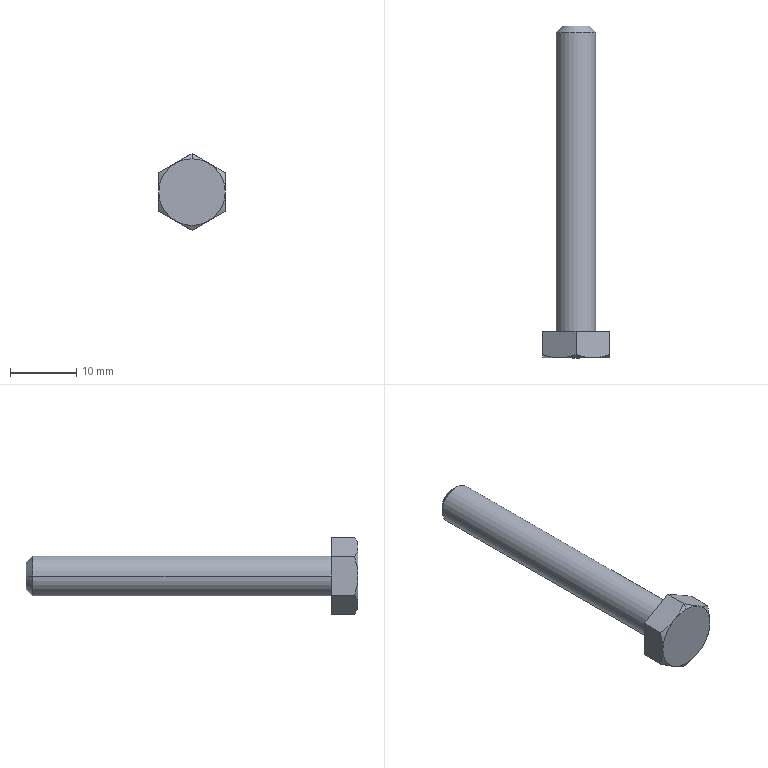Part | STEP file | 11-NEZI-M6x40L_MC01-S311 | 1 solid | 20 faces | box 10 x 50 x 11.547 mm | volume 1637 mm3 | cone 9 | plane 9 | cylinder 2 | commonest cylinder face diameters 6 x2
STEP:
#1=CARTESIAN_POINT('',(-2.,50.,0.));
#2=VERTEX_POINT('',#1);
#3=CARTESIAN_POINT('',(2.,50.,0.));
#4=VERTEX_POINT('',#3);
#5=CARTESIAN_POINT('',(0.,50.,0.));
#6=DIRECTION('',(0.,1.,0.));
#7=DIRECTION('',(-1.,0.,0.));
#8=AXIS2_PLACEMENT_3D('',#5,#6,#7);
#9=CIRCLE('',#8,2.);
#10=EDGE_CURVE('',#2,#4,#9,.T.);
#11=ORIENTED_EDGE('',*,*,#10,.F.);
#12=CARTESIAN_POINT('',(-3.,49.,0.));
#13=VERTEX_POINT('',#12);
#14=CARTESIAN_POINT('',(-2.,50.,0.));
#15=DIRECTION('',(-0.7071,-0.7071,0.));
#16=VECTOR('',#15,1000.);
#17=LINE('',#14,#16);
#18=EDGE_CURVE('',#2,#13,#17,.T.);
#19=ORIENTED_EDGE('',*,*,#18,.T.);
#20=CARTESIAN_POINT('',(3.,49.,0.));
#21=VERTEX_POINT('',#20);
#22=CARTESIAN_POINT('',(0.,49.,0.));
#23=DIRECTION('',(0.,-1.,0.));
#24=DIRECTION('',(-1.,0.,0.));
#25=AXIS2_PLACEMENT_3D('',#22,#23,#24);
#26=CIRCLE('',#25,3.);
#27=EDGE_CURVE('',#21,#13,#26,.T.);
#28=ORIENTED_EDGE('',*,*,#27,.F.);
#29=CARTESIAN_POINT('',(2.,50.,0.));
#30=DIRECTION('',(0.7071,-0.7071,0.));
#31=VECTOR('',#30,1000.);
#32=LINE('',#29,#31);
#33=EDGE_CURVE('',#4,#21,#32,.T.);
#34=ORIENTED_EDGE('',*,*,#33,.F.);
#35=EDGE_LOOP('',(#11,#19,#28,#34));
#36=FACE_OUTER_BOUND('',#35,.T.);
#37=CARTESIAN_POINT('',(0.,50.,0.));
#38=DIRECTION('',(0.,-1.,0.));
#39=DIRECTION('',(1.,0.,0.));
#40=AXIS2_PLACEMENT_3D('',#37,#38,#39);
#41=CONICAL_SURFACE('',#40,2.,0.7854);
#42=ADVANCED_FACE('',(#36),#41,.T.);
#43=CARTESIAN_POINT('',(0.,0.,5.));
#44=VERTEX_POINT('',#43);
#45=CARTESIAN_POINT('',(-2.5,0.,4.33));
#46=VERTEX_POINT('',#45);
#47=CARTESIAN_POINT('',(0.,0.,0.));
#48=DIRECTION('',(0.,-1.,0.));
#49=DIRECTION('',(1.,0.,0.));
#50=AXIS2_PLACEMENT_3D('',#47,#48,#49);
#51=CIRCLE('',#50,5.);
#52=EDGE_CURVE('',#44,#46,#51,.T.);
#53=ORIENTED_EDGE('',*,*,#52,.F.);
#54=CARTESIAN_POINT('',(0.,0.5,5.774));
#55=VERTEX_POINT('',#54);
#56=CARTESIAN_POINT('',(0.,0.,5.));
#57=DIRECTION('',(0.,0.5429,0.8398));
#58=VECTOR('',#57,1000.);
#59=LINE('',#56,#58);
#60=EDGE_CURVE('',#44,#55,#59,.T.);
#61=ORIENTED_EDGE('',*,*,#60,.T.);
#62=CARTESIAN_POINT('',(0.,0.5,5.774));
#63=CARTESIAN_POINT('',(-0.8145,0.196,5.303));
#64=CARTESIAN_POINT('',(-1.644,0.,4.824));
#65=CARTESIAN_POINT('',(-2.5,0.,4.33));
#66=B_SPLINE_CURVE_WITH_KNOTS('',3,(#62,#63,#64,#65),.UNSPECIFIED.,.F.,.F.,(4,4),(0.00000024,0.00293),.UNSPECIFIED.);
#67=EDGE_CURVE('',#55,#46,#66,.T.);
#68=ORIENTED_EDGE('',*,*,#67,.T.);
#69=EDGE_LOOP('',(#53,#61,#68));
#70=FACE_OUTER_BOUND('',#69,.T.);
#71=CARTESIAN_POINT('',(0.,0.,0.));
#72=DIRECTION('',(0.,1.,0.));
#73=DIRECTION('',(0.,0.,1.));
#74=AXIS2_PLACEMENT_3D('',#71,#72,#73);
#75=CONICAL_SURFACE('',#74,5.,0.9969);
#76=ADVANCED_FACE('',(#70),#75,.T.);
#77=CARTESIAN_POINT('',(-3.,4.,0.));
#78=VERTEX_POINT('',#77);
#79=CARTESIAN_POINT('',(3.,4.,0.));
#80=VERTEX_POINT('',#79);
#81=CARTESIAN_POINT('',(0.,4.,0.));
#82=DIRECTION('',(0.,1.,0.));
#83=DIRECTION('',(-1.,0.,0.));
#84=AXIS2_PLACEMENT_3D('',#81,#82,#83);
#85=CIRCLE('',#84,3.);
#86=EDGE_CURVE('',#78,#80,#85,.T.);
#87=ORIENTED_EDGE('',*,*,#86,.T.);
#88=CARTESIAN_POINT('',(3.,50.,0.));
#89=DIRECTION('',(0.,1.,0.));
#90=VECTOR('',#89,1000.);
#91=LINE('',#88,#90);
#92=EDGE_CURVE('',#80,#21,#91,.T.);
#93=ORIENTED_EDGE('',*,*,#92,.T.);
#94=ORIENTED_EDGE('',*,*,#27,.T.);
#95=CARTESIAN_POINT('',(-3.,50.,0.));
#96=DIRECTION('',(0.,1.,0.));
#97=VECTOR('',#96,1000.);
#98=LINE('',#95,#97);
#99=EDGE_CURVE('',#78,#13,#98,.T.);
#100=ORIENTED_EDGE('',*,*,#99,.F.);
#101=EDGE_LOOP('',(#87,#93,#94,#100));
#102=FACE_OUTER_BOUND('',#101,.T.);
#103=CARTESIAN_POINT('',(0.,50.,0.));
#104=DIRECTION('',(0.,1.,0.));
#105=DIRECTION('',(-1.,0.,0.));
#106=AXIS2_PLACEMENT_3D('',#103,#104,#105);
#107=CYLINDRICAL_SURFACE('',#106,3.);
#108=ADVANCED_FACE('',(#102),#107,.T.);
#109=CARTESIAN_POINT('',(0.,0.5,-5.774));
#110=VERTEX_POINT('',#109);
#111=CARTESIAN_POINT('',(2.5,0.,-4.33));
#112=VERTEX_POINT('',#111);
#113=CARTESIAN_POINT('',(0.,0.5,-5.774));
#114=CARTESIAN_POINT('',(0.8145,0.196,-5.303));
#115=CARTESIAN_POINT('',(1.644,0.,-4.824));
#116=CARTESIAN_POINT('',(2.5,0.,-4.33));
#117=B_SPLINE_CURVE_WITH_KNOTS('',3,(#113,#114,#115,#116),.UNSPECIFIED.,.F.,.F.,(4,4),(0.00000024,0.00293),.UNSPECIFIED.);
#118=EDGE_CURVE('',#110,#112,#117,.T.);
#119=ORIENTED_EDGE('',*,*,#118,.F.);
#120=CARTESIAN_POINT('',(0.,4.,-5.774));
#121=VERTEX_POINT('',#120);
#122=CARTESIAN_POINT('',(0.,50.,-5.774));
#123=DIRECTION('',(0.,-1.,0.));
#124=VECTOR('',#123,1000.);
#125=LINE('',#122,#124);
#126=EDGE_CURVE('',#121,#110,#125,.T.);
#127=ORIENTED_EDGE('',*,*,#126,.F.);
#128=CARTESIAN_POINT('',(5.,4.,-2.887));
#129=VERTEX_POINT('',#128);
#130=CARTESIAN_POINT('',(-3.125,4.,-7.578));
#131=DIRECTION('',(0.866,0.,0.5));
#132=VECTOR('',#131,1000.);
#133=LINE('',#130,#132);
#134=EDGE_CURVE('',#121,#129,#133,.T.);
#135=ORIENTED_EDGE('',*,*,#134,.T.);
#136=CARTESIAN_POINT('',(5.,0.5,-2.887));
#137=VERTEX_POINT('',#136);
#138=CARTESIAN_POINT('',(5.,50.,-2.887));
#139=DIRECTION('',(0.,-1.,0.));
#140=VECTOR('',#139,1000.);
#141=LINE('',#138,#140);
#142=EDGE_CURVE('',#129,#137,#141,.T.);
#143=ORIENTED_EDGE('',*,*,#142,.T.);
#144=CARTESIAN_POINT('',(2.5,0.,-4.33));
#145=CARTESIAN_POINT('',(2.713,0.,-4.207));
#146=CARTESIAN_POINT('',(2.927,0.01194,-4.083));
#147=CARTESIAN_POINT('',(3.35,0.05801,-3.839));
#148=CARTESIAN_POINT('',(3.56,0.09207,-3.718));
#149=CARTESIAN_POINT('',(4.184,0.223,-3.358));
#150=CARTESIAN_POINT('',(4.594,0.3486,-3.121));
#151=CARTESIAN_POINT('',(5.,0.5,-2.887));
#152=B_SPLINE_CURVE_WITH_KNOTS('',3,(#144,#145,#146,#147,#148,#149,#150,#151),.UNSPECIFIED.,.F.,.F.,(4,2,2,4),(0.00293,0.003658,0.004386,0.005842),.UNSPECIFIED.);
#153=EDGE_CURVE('',#112,#137,#152,.T.);
#154=ORIENTED_EDGE('',*,*,#153,.F.);
#155=EDGE_LOOP('',(#119,#127,#135,#143,#154));
#156=FACE_OUTER_BOUND('',#155,.T.);
#157=CARTESIAN_POINT('',(5.,50.,-2.887));
#158=DIRECTION('',(-0.5,0.,0.866));
#159=DIRECTION('',(0.866,0.,0.5));
#160=AXIS2_PLACEMENT_3D('',#157,#158,#159);
#161=PLANE('',#160);
#162=ADVANCED_FACE('',(#156),#161,.F.);
#163=CARTESIAN_POINT('',(-5.,0.5,-2.887));
#164=VERTEX_POINT('',#163);
#165=CARTESIAN_POINT('',(-2.5,0.,-4.33));
#166=VERTEX_POINT('',#165);
#167=CARTESIAN_POINT('',(-5.,0.5,-2.887));
#168=CARTESIAN_POINT('',(-4.185,0.196,-3.357));
#169=CARTESIAN_POINT('',(-3.356,0.,-3.836));
#170=CARTESIAN_POINT('',(-2.5,0.,-4.33));
#171=B_SPLINE_CURVE_WITH_KNOTS('',3,(#167,#168,#169,#170),.UNSPECIFIED.,.F.,.F.,(4,4),(0.00000024,0.00293),.UNSPECIFIED.);
#172=EDGE_CURVE('',#164,#166,#171,.T.);
#173=ORIENTED_EDGE('',*,*,#172,.F.);
#174=CARTESIAN_POINT('',(-5.,4.,-2.887));
#175=VERTEX_POINT('',#174);
#176=CARTESIAN_POINT('',(-5.,50.,-2.887));
#177=DIRECTION('',(0.,-1.,0.));
#178=VECTOR('',#177,1000.);
#179=LINE('',#176,#178);
#180=EDGE_CURVE('',#175,#164,#179,.T.);
#181=ORIENTED_EDGE('',*,*,#180,.F.);
#182=CARTESIAN_POINT('',(-8.125,4.,-1.083));
#183=DIRECTION('',(0.866,0.,-0.5));
#184=VECTOR('',#183,1000.);
#185=LINE('',#182,#184);
#186=EDGE_CURVE('',#175,#121,#185,.T.);
#187=ORIENTED_EDGE('',*,*,#186,.T.);
#188=ORIENTED_EDGE('',*,*,#126,.T.);
#189=CARTESIAN_POINT('',(-2.5,0.,-4.33));
#190=CARTESIAN_POINT('',(-2.287,0.,-4.453));
#191=CARTESIAN_POINT('',(-2.073,0.01194,-4.577));
#192=CARTESIAN_POINT('',(-1.65,0.05801,-4.821));
#193=CARTESIAN_POINT('',(-1.44,0.09207,-4.942));
#194=CARTESIAN_POINT('',(-0.8158,0.223,-5.303));
#195=CARTESIAN_POINT('',(-0.4058,0.3486,-5.539));
#196=CARTESIAN_POINT('',(0.,0.5,-5.774));
#197=B_SPLINE_CURVE_WITH_KNOTS('',3,(#189,#190,#191,#192,#193,#194,#195,#196),.UNSPECIFIED.,.F.,.F.,(4,2,2,4),(0.00293,0.003658,0.004386,0.005842),.UNSPECIFIED.);
#198=EDGE_CURVE('',#166,#110,#197,.T.);
#199=ORIENTED_EDGE('',*,*,#198,.F.);
#200=EDGE_LOOP('',(#173,#181,#187,#188,#199));
#201=FACE_OUTER_BOUND('',#200,.T.);
#202=CARTESIAN_POINT('',(0.,50.,-5.774));
#203=DIRECTION('',(0.5,0.,0.866));
#204=DIRECTION('',(0.866,0.,-0.5));
#205=AXIS2_PLACEMENT_3D('',#202,#203,#204);
#206=PLANE('',#205);
#207=ADVANCED_FACE('',(#201),#206,.F.);
#208=CARTESIAN_POINT('',(-5.,0.5,2.887));
#209=VERTEX_POINT('',#208);
#210=CARTESIAN_POINT('',(-5.,0.,0.));
#211=VERTEX_POINT('',#210);
#212=CARTESIAN_POINT('',(-5.,0.5,2.887));
#213=CARTESIAN_POINT('',(-5.,0.3499,2.422));
#214=CARTESIAN_POINT('',(-5.,0.2243,1.951));
#215=CARTESIAN_POINT('',(-5.,0.04855,0.9855));
#216=CARTESIAN_POINT('',(-5.,0.,0.4886));
#217=CARTESIAN_POINT('',(-5.,0.,0.));
#218=B_SPLINE_CURVE_WITH_KNOTS('',3,(#212,#213,#214,#215,#216,#217),.UNSPECIFIED.,.F.,.F.,(4,2,4),(0.001661,0.003125,0.004588),.UNSPECIFIED.);
#219=EDGE_CURVE('',#209,#211,#218,.T.);
#220=ORIENTED_EDGE('',*,*,#219,.F.);
#221=CARTESIAN_POINT('',(-5.,4.,2.887));
#222=VERTEX_POINT('',#221);
#223=CARTESIAN_POINT('',(-5.,50.,2.887));
#224=DIRECTION('',(0.,-1.,0.));
#225=VECTOR('',#224,1000.);
#226=LINE('',#223,#225);
#227=EDGE_CURVE('',#222,#209,#226,.T.);
#228=ORIENTED_EDGE('',*,*,#227,.F.);
#229=CARTESIAN_POINT('',(-5.,4.,0.));
#230=DIRECTION('',(0.,0.,-1.));
#231=VECTOR('',#230,1000.);
#232=LINE('',#229,#231);
#233=EDGE_CURVE('',#222,#175,#232,.T.);
#234=ORIENTED_EDGE('',*,*,#233,.T.);
#235=ORIENTED_EDGE('',*,*,#180,.T.);
#236=CARTESIAN_POINT('',(-5.,0.,0.));
#237=CARTESIAN_POINT('',(-5.,0.,-0.4892));
#238=CARTESIAN_POINT('',(-5.,0.0472,-0.9746));
#239=CARTESIAN_POINT('',(-5.,0.2216,-1.939));
#240=CARTESIAN_POINT('',(-5.,0.349,-2.42));
#241=CARTESIAN_POINT('',(-5.,0.5,-2.887));
#242=B_SPLINE_CURVE_WITH_KNOTS('',3,(#236,#237,#238,#239,#240,#241),.UNSPECIFIED.,.F.,.F.,(4,2,4),(0.004588,0.006054,0.00752),.UNSPECIFIED.);
#243=EDGE_CURVE('',#211,#164,#242,.T.);
#244=ORIENTED_EDGE('',*,*,#243,.F.);
#245=EDGE_LOOP('',(#220,#228,#234,#235,#244));
#246=FACE_OUTER_BOUND('',#245,.T.);
#247=CARTESIAN_POINT('',(-5.,50.,-2.887));
#248=DIRECTION('',(1.,0.,0.));
#249=DIRECTION('',(0.,0.,-1.));
#250=AXIS2_PLACEMENT_3D('',#247,#248,#249);
#251=PLANE('',#250);
#252=ADVANCED_FACE('',(#246),#251,.F.);
#253=ORIENTED_EDGE('',*,*,#67,.F.);
#254=CARTESIAN_POINT('',(0.,4.,5.774));
#255=VERTEX_POINT('',#254);
#256=CARTESIAN_POINT('',(0.,50.,5.774));
#257=DIRECTION('',(0.,-1.,0.));
#258=VECTOR('',#257,1000.);
#259=LINE('',#256,#258);
#260=EDGE_CURVE('',#255,#55,#259,.T.);
#261=ORIENTED_EDGE('',*,*,#260,.F.);
#262=CARTESIAN_POINT('',(-8.125,4.,1.083));
#263=DIRECTION('',(-0.866,0.,-0.5));
#264=VECTOR('',#263,1000.);
#265=LINE('',#262,#264);
#266=EDGE_CURVE('',#255,#222,#265,.T.);
#267=ORIENTED_EDGE('',*,*,#266,.T.);
#268=ORIENTED_EDGE('',*,*,#227,.T.);
#269=CARTESIAN_POINT('',(-2.5,0.,4.33));
#270=CARTESIAN_POINT('',(-2.713,0.,4.207));
#271=CARTESIAN_POINT('',(-2.927,0.01194,4.083));
#272=CARTESIAN_POINT('',(-3.35,0.05801,3.839));
#273=CARTESIAN_POINT('',(-3.56,0.09207,3.718));
#274=CARTESIAN_POINT('',(-4.184,0.223,3.358));
#275=CARTESIAN_POINT('',(-4.594,0.3486,3.121));
#276=CARTESIAN_POINT('',(-5.,0.5,2.887));
#277=B_SPLINE_CURVE_WITH_KNOTS('',3,(#269,#270,#271,#272,#273,#274,#275,#276),.UNSPECIFIED.,.F.,.F.,(4,2,2,4),(0.00293,0.003658,0.004386,0.005842),.UNSPECIFIED.);
#278=EDGE_CURVE('',#46,#209,#277,.T.);
#279=ORIENTED_EDGE('',*,*,#278,.F.);
#280=EDGE_LOOP('',(#253,#261,#267,#268,#279));
#281=FACE_OUTER_BOUND('',#280,.T.);
#282=CARTESIAN_POINT('',(-5.,50.,2.887));
#283=DIRECTION('',(0.5,0.,-0.866));
#284=DIRECTION('',(-0.866,0.,-0.5));
#285=AXIS2_PLACEMENT_3D('',#282,#283,#284);
#286=PLANE('',#285);
#287=ADVANCED_FACE('',(#281),#286,.F.);
#288=CARTESIAN_POINT('',(5.,0.5,2.887));
#289=VERTEX_POINT('',#288);
#290=CARTESIAN_POINT('',(2.5,0.,4.33));
#291=VERTEX_POINT('',#290);
#292=CARTESIAN_POINT('',(5.,0.5,2.887));
#293=CARTESIAN_POINT('',(4.185,0.196,3.357));
#294=CARTESIAN_POINT('',(3.356,0.,3.836));
#295=CARTESIAN_POINT('',(2.5,0.,4.33));
#296=B_SPLINE_CURVE_WITH_KNOTS('',3,(#292,#293,#294,#295),.UNSPECIFIED.,.F.,.F.,(4,4),(0.00000024,0.00293),.UNSPECIFIED.);
#297=EDGE_CURVE('',#289,#291,#296,.T.);
#298=ORIENTED_EDGE('',*,*,#297,.F.);
#299=CARTESIAN_POINT('',(5.,4.,2.887));
#300=VERTEX_POINT('',#299);
#301=CARTESIAN_POINT('',(5.,50.,2.887));
#302=DIRECTION('',(0.,-1.,0.));
#303=VECTOR('',#302,1000.);
#304=LINE('',#301,#303);
#305=EDGE_CURVE('',#300,#289,#304,.T.);
#306=ORIENTED_EDGE('',*,*,#305,.F.);
#307=CARTESIAN_POINT('',(-3.125,4.,7.578));
#308=DIRECTION('',(-0.866,0.,0.5));
#309=VECTOR('',#308,1000.);
#310=LINE('',#307,#309);
#311=EDGE_CURVE('',#300,#255,#310,.T.);
#312=ORIENTED_EDGE('',*,*,#311,.T.);
#313=ORIENTED_EDGE('',*,*,#260,.T.);
#314=CARTESIAN_POINT('',(2.5,0.,4.33));
#315=CARTESIAN_POINT('',(2.287,0.,4.453));
#316=CARTESIAN_POINT('',(2.073,0.01194,4.577));
#317=CARTESIAN_POINT('',(1.65,0.05801,4.821));
#318=CARTESIAN_POINT('',(1.44,0.09207,4.942));
#319=CARTESIAN_POINT('',(0.8158,0.223,5.303));
#320=CARTESIAN_POINT('',(0.4058,0.3486,5.539));
#321=CARTESIAN_POINT('',(0.,0.5,5.774));
#322=B_SPLINE_CURVE_WITH_KNOTS('',3,(#314,#315,#316,#317,#318,#319,#320,#321),.UNSPECIFIED.,.F.,.F.,(4,2,2,4),(0.00293,0.003658,0.004386,0.005842),.UNSPECIFIED.);
#323=EDGE_CURVE('',#291,#55,#322,.T.);
#324=ORIENTED_EDGE('',*,*,#323,.F.);
#325=EDGE_LOOP('',(#298,#306,#312,#313,#324));
#326=FACE_OUTER_BOUND('',#325,.T.);
#327=CARTESIAN_POINT('',(0.,50.,5.774));
#328=DIRECTION('',(-0.5,0.,-0.866));
#329=DIRECTION('',(-0.866,0.,0.5));
#330=AXIS2_PLACEMENT_3D('',#327,#328,#329);
#331=PLANE('',#330);
#332=ADVANCED_FACE('',(#326),#331,.F.);
#333=CARTESIAN_POINT('',(5.,0.,0.));
#334=VERTEX_POINT('',#333);
#335=CARTESIAN_POINT('',(5.,0.5,-2.887));
#336=CARTESIAN_POINT('',(5.,0.349,-2.42));
#337=CARTESIAN_POINT('',(5.,0.2216,-1.939));
#338=CARTESIAN_POINT('',(5.,0.0472,-0.9746));
#339=CARTESIAN_POINT('',(5.,0.,-0.4892));
#340=CARTESIAN_POINT('',(5.,0.,0.));
#341=B_SPLINE_CURVE_WITH_KNOTS('',3,(#335,#336,#337,#338,#339,#340),.UNSPECIFIED.,.F.,.F.,(4,2,4),(0.0049,0.006366,0.007833),.UNSPECIFIED.);
#342=EDGE_CURVE('',#137,#334,#341,.T.);
#343=ORIENTED_EDGE('',*,*,#342,.F.);
#344=ORIENTED_EDGE('',*,*,#142,.F.);
#345=CARTESIAN_POINT('',(5.,4.,0.));
#346=DIRECTION('',(0.,0.,1.));
#347=VECTOR('',#346,1000.);
#348=LINE('',#345,#347);
#349=EDGE_CURVE('',#129,#300,#348,.T.);
#350=ORIENTED_EDGE('',*,*,#349,.T.);
#351=ORIENTED_EDGE('',*,*,#305,.T.);
#352=CARTESIAN_POINT('',(5.,0.,0.));
#353=CARTESIAN_POINT('',(5.,0.,0.4886));
#354=CARTESIAN_POINT('',(5.,0.04855,0.9855));
#355=CARTESIAN_POINT('',(5.,0.2243,1.951));
#356=CARTESIAN_POINT('',(5.,0.3499,2.422));
#357=CARTESIAN_POINT('',(5.,0.5,2.887));
#358=B_SPLINE_CURVE_WITH_KNOTS('',3,(#352,#353,#354,#355,#356,#357),.UNSPECIFIED.,.F.,.F.,(4,2,4),(0.007833,0.009297,0.01076),.UNSPECIFIED.);
#359=EDGE_CURVE('',#334,#289,#358,.T.);
#360=ORIENTED_EDGE('',*,*,#359,.F.);
#361=EDGE_LOOP('',(#343,#344,#350,#351,#360));
#362=FACE_OUTER_BOUND('',#361,.T.);
#363=CARTESIAN_POINT('',(5.,50.,2.887));
#364=DIRECTION('',(-1.,0.,0.));
#365=DIRECTION('',(0.,0.,1.));
#366=AXIS2_PLACEMENT_3D('',#363,#364,#365);
#367=PLANE('',#366);
#368=ADVANCED_FACE('',(#362),#367,.F.);
#369=ORIENTED_EDGE('',*,*,#134,.F.);
#370=ORIENTED_EDGE('',*,*,#186,.F.);
#371=ORIENTED_EDGE('',*,*,#233,.F.);
#372=ORIENTED_EDGE('',*,*,#266,.F.);
#373=ORIENTED_EDGE('',*,*,#311,.F.);
#374=ORIENTED_EDGE('',*,*,#349,.F.);
#375=EDGE_LOOP('',(#369,#370,#371,#372,#373,#374));
#376=FACE_OUTER_BOUND('',#375,.T.);
#377=ORIENTED_EDGE('',*,*,#86,.F.);
#378=CARTESIAN_POINT('',(0.,4.,0.));
#379=DIRECTION('',(0.,1.,0.));
#380=DIRECTION('',(-1.,0.,0.));
#381=AXIS2_PLACEMENT_3D('',#378,#379,#380);
#382=CIRCLE('',#381,3.);
#383=EDGE_CURVE('',#80,#78,#382,.T.);
#384=ORIENTED_EDGE('',*,*,#383,.F.);
#385=EDGE_LOOP('',(#377,#384));
#386=FACE_BOUND('',#385,.T.);
#387=CARTESIAN_POINT('',(-7.5,4.,0.));
#388=DIRECTION('',(0.,1.,0.));
#389=DIRECTION('',(-1.,0.,0.));
#390=AXIS2_PLACEMENT_3D('',#387,#388,#389);
#391=PLANE('',#390);
#392=ADVANCED_FACE('',(#376,#386),#391,.T.);
#393=ORIENTED_EDGE('',*,*,#92,.F.);
#394=ORIENTED_EDGE('',*,*,#383,.T.);
#395=ORIENTED_EDGE('',*,*,#99,.T.);
#396=CARTESIAN_POINT('',(0.,49.,0.));
#397=DIRECTION('',(0.,-1.,0.));
#398=DIRECTION('',(-1.,0.,0.));
#399=AXIS2_PLACEMENT_3D('',#396,#397,#398);
#400=CIRCLE('',#399,3.);
#401=EDGE_CURVE('',#13,#21,#400,.T.);
#402=ORIENTED_EDGE('',*,*,#401,.T.);
#403=EDGE_LOOP('',(#393,#394,#395,#402));
#404=FACE_OUTER_BOUND('',#403,.T.);
#405=CARTESIAN_POINT('',(0.,50.,0.));
#406=DIRECTION('',(0.,1.,0.));
#407=DIRECTION('',(-1.,0.,0.));
#408=AXIS2_PLACEMENT_3D('',#405,#406,#407);
#409=CYLINDRICAL_SURFACE('',#408,3.);
#410=ADVANCED_FACE('',(#404),#409,.T.);
#411=CARTESIAN_POINT('',(0.,50.,0.));
#412=DIRECTION('',(0.,1.,0.));
#413=DIRECTION('',(-1.,0.,0.));
#414=AXIS2_PLACEMENT_3D('',#411,#412,#413);
#415=CIRCLE('',#414,2.);
#416=EDGE_CURVE('',#4,#2,#415,.T.);
#417=ORIENTED_EDGE('',*,*,#416,.T.);
#418=ORIENTED_EDGE('',*,*,#10,.T.);
#419=EDGE_LOOP('',(#417,#418));
#420=FACE_OUTER_BOUND('',#419,.T.);
#421=CARTESIAN_POINT('',(-3.,50.,0.));
#422=DIRECTION('',(0.,1.,0.));
#423=DIRECTION('',(-1.,0.,0.));
#424=AXIS2_PLACEMENT_3D('',#421,#422,#423);
#425=PLANE('',#424);
#426=ADVANCED_FACE('',(#420),#425,.T.);
#427=ORIENTED_EDGE('',*,*,#153,.T.);
#428=ORIENTED_EDGE('',*,*,#342,.T.);
#429=CARTESIAN_POINT('',(0.,0.,0.));
#430=DIRECTION('',(0.,-1.,0.));
#431=DIRECTION('',(0.,0.,-1.));
#432=AXIS2_PLACEMENT_3D('',#429,#430,#431);
#433=CIRCLE('',#432,5.);
#434=EDGE_CURVE('',#112,#334,#433,.T.);
#435=ORIENTED_EDGE('',*,*,#434,.F.);
#436=EDGE_LOOP('',(#427,#428,#435));
#437=FACE_OUTER_BOUND('',#436,.T.);
#438=CARTESIAN_POINT('',(0.,0.,0.));
#439=DIRECTION('',(0.,1.,0.));
#440=DIRECTION('',(0.,0.,1.));
#441=AXIS2_PLACEMENT_3D('',#438,#439,#440);
#442=CONICAL_SURFACE('',#441,5.,0.9969);
#443=ADVANCED_FACE('',(#437),#442,.T.);
#444=ORIENTED_EDGE('',*,*,#198,.T.);
#445=ORIENTED_EDGE('',*,*,#118,.T.);
#446=CARTESIAN_POINT('',(0.,0.,0.));
#447=DIRECTION('',(0.,-1.,0.));
#448=DIRECTION('',(1.,0.,0.));
#449=AXIS2_PLACEMENT_3D('',#446,#447,#448);
#450=CIRCLE('',#449,5.);
#451=EDGE_CURVE('',#166,#112,#450,.T.);
#452=ORIENTED_EDGE('',*,*,#451,.F.);
#453=EDGE_LOOP('',(#444,#445,#452));
#454=FACE_OUTER_BOUND('',#453,.T.);
#455=CARTESIAN_POINT('',(0.,0.,0.));
#456=DIRECTION('',(0.,1.,0.));
#457=DIRECTION('',(0.,0.,1.));
#458=AXIS2_PLACEMENT_3D('',#455,#456,#457);
#459=CONICAL_SURFACE('',#458,5.,0.9969);
#460=ADVANCED_FACE('',(#454),#459,.T.);
#461=ORIENTED_EDGE('',*,*,#243,.T.);
#462=ORIENTED_EDGE('',*,*,#172,.T.);
#463=CARTESIAN_POINT('',(0.,0.,0.));
#464=DIRECTION('',(0.,-1.,0.));
#465=DIRECTION('',(1.,0.,0.));
#466=AXIS2_PLACEMENT_3D('',#463,#464,#465);
#467=CIRCLE('',#466,5.);
#468=EDGE_CURVE('',#211,#166,#467,.T.);
#469=ORIENTED_EDGE('',*,*,#468,.F.);
#470=EDGE_LOOP('',(#461,#462,#469));
#471=FACE_OUTER_BOUND('',#470,.T.);
#472=CARTESIAN_POINT('',(0.,0.,0.));
#473=DIRECTION('',(0.,1.,0.));
#474=DIRECTION('',(0.,0.,1.));
#475=AXIS2_PLACEMENT_3D('',#472,#473,#474);
#476=CONICAL_SURFACE('',#475,5.,0.9969);
#477=ADVANCED_FACE('',(#471),#476,.T.);
#478=ORIENTED_EDGE('',*,*,#219,.T.);
#479=CARTESIAN_POINT('',(0.,0.,0.));
#480=DIRECTION('',(0.,-1.,0.));
#481=DIRECTION('',(1.,0.,0.));
#482=AXIS2_PLACEMENT_3D('',#479,#480,#481);
#483=CIRCLE('',#482,5.);
#484=EDGE_CURVE('',#46,#211,#483,.T.);
#485=ORIENTED_EDGE('',*,*,#484,.F.);
#486=ORIENTED_EDGE('',*,*,#278,.T.);
#487=EDGE_LOOP('',(#478,#485,#486));
#488=FACE_OUTER_BOUND('',#487,.T.);
#489=CARTESIAN_POINT('',(0.,0.,0.));
#490=DIRECTION('',(0.,1.,0.));
#491=DIRECTION('',(0.,0.,1.));
#492=AXIS2_PLACEMENT_3D('',#489,#490,#491);
#493=CONICAL_SURFACE('',#492,5.,0.9969);
#494=ADVANCED_FACE('',(#488),#493,.T.);
#495=ORIENTED_EDGE('',*,*,#60,.F.);
#496=CARTESIAN_POINT('',(0.,0.,0.));
#497=DIRECTION('',(0.,-1.,0.));
#498=DIRECTION('',(1.,0.,0.));
#499=AXIS2_PLACEMENT_3D('',#496,#497,#498);
#500=CIRCLE('',#499,5.);
#501=EDGE_CURVE('',#291,#44,#500,.T.);
#502=ORIENTED_EDGE('',*,*,#501,.F.);
#503=ORIENTED_EDGE('',*,*,#323,.T.);
#504=EDGE_LOOP('',(#495,#502,#503));
#505=FACE_OUTER_BOUND('',#504,.T.);
#506=CARTESIAN_POINT('',(0.,0.,0.));
#507=DIRECTION('',(0.,1.,0.));
#508=DIRECTION('',(0.,0.,1.));
#509=AXIS2_PLACEMENT_3D('',#506,#507,#508);
#510=CONICAL_SURFACE('',#509,5.,0.9969);
#511=ADVANCED_FACE('',(#505),#510,.T.);
#512=ORIENTED_EDGE('',*,*,#297,.T.);
#513=CARTESIAN_POINT('',(0.,0.,0.));
#514=DIRECTION('',(0.,-1.,0.));
#515=DIRECTION('',(1.,0.,0.));
#516=AXIS2_PLACEMENT_3D('',#513,#514,#515);
#517=CIRCLE('',#516,5.);
#518=EDGE_CURVE('',#334,#291,#517,.T.);
#519=ORIENTED_EDGE('',*,*,#518,.F.);
#520=ORIENTED_EDGE('',*,*,#359,.T.);
#521=EDGE_LOOP('',(#512,#519,#520));
#522=FACE_OUTER_BOUND('',#521,.T.);
#523=CARTESIAN_POINT('',(0.,0.,0.));
#524=DIRECTION('',(0.,1.,0.));
#525=DIRECTION('',(0.,0.,1.));
#526=AXIS2_PLACEMENT_3D('',#523,#524,#525);
#527=CONICAL_SURFACE('',#526,5.,0.9969);
#528=ADVANCED_FACE('',(#522),#527,.T.);
#529=ORIENTED_EDGE('',*,*,#434,.T.);
#530=ORIENTED_EDGE('',*,*,#518,.T.);
#531=ORIENTED_EDGE('',*,*,#501,.T.);
#532=ORIENTED_EDGE('',*,*,#52,.T.);
#533=ORIENTED_EDGE('',*,*,#484,.T.);
#534=ORIENTED_EDGE('',*,*,#468,.T.);
#535=ORIENTED_EDGE('',*,*,#451,.T.);
#536=EDGE_LOOP('',(#529,#530,#531,#532,#533,#534,#535));
#537=FACE_OUTER_BOUND('',#536,.T.);
#538=CARTESIAN_POINT('',(0.,0.,0.));
#539=DIRECTION('',(0.,-1.,0.));
#540=DIRECTION('',(1.,0.,0.));
#541=AXIS2_PLACEMENT_3D('',#538,#539,#540);
#542=PLANE('',#541);
#543=ADVANCED_FACE('',(#537),#542,.T.);
#544=ORIENTED_EDGE('',*,*,#18,.F.);
#545=ORIENTED_EDGE('',*,*,#416,.F.);
#546=ORIENTED_EDGE('',*,*,#33,.T.);
#547=ORIENTED_EDGE('',*,*,#401,.F.);
#548=EDGE_LOOP('',(#544,#545,#546,#547));
#549=FACE_OUTER_BOUND('',#548,.T.);
#550=CARTESIAN_POINT('',(0.,50.,0.));
#551=DIRECTION('',(0.,-1.,0.));
#552=DIRECTION('',(1.,0.,0.));
#553=AXIS2_PLACEMENT_3D('',#550,#551,#552);
#554=CONICAL_SURFACE('',#553,2.,0.7854);
#555=ADVANCED_FACE('',(#549),#554,.T.);
#556=CLOSED_SHELL('',(#42,#76,#108,#162,#207,#252,#287,#332,#368,#392,#410,#426,#443,#460,#477,#494,#511,#528,#543,#555));
#557=MANIFOLD_SOLID_BREP('',#556);
#558=CARTESIAN_POINT('',(0.,0.,0.));
#559=DIRECTION('',(0.,0.,1.));
#560=DIRECTION('',(1.,0.,0.));
#561=AXIS2_PLACEMENT_3D('',#558,#559,#560);
#562=(LENGTH_UNIT()NAMED_UNIT(*)SI_UNIT(.MILLI.,.METRE.));
#563=UNCERTAINTY_MEASURE_WITH_UNIT(LENGTH_MEASURE(0.00001),#562,'','');
#564=(NAMED_UNIT(*)PLANE_ANGLE_UNIT()SI_UNIT($,.RADIAN.));
#565=(NAMED_UNIT(*)SI_UNIT($,.STERADIAN.)SOLID_ANGLE_UNIT());
#566=(GEOMETRIC_REPRESENTATION_CONTEXT(3)GLOBAL_UNCERTAINTY_ASSIGNED_CONTEXT((#563))GLOBAL_UNIT_ASSIGNED_CONTEXT((#562,#564,#565))REPRESENTATION_CONTEXT('',''));
#567=ADVANCED_BREP_SHAPE_REPRESENTATION('',(#557,#561),#566);